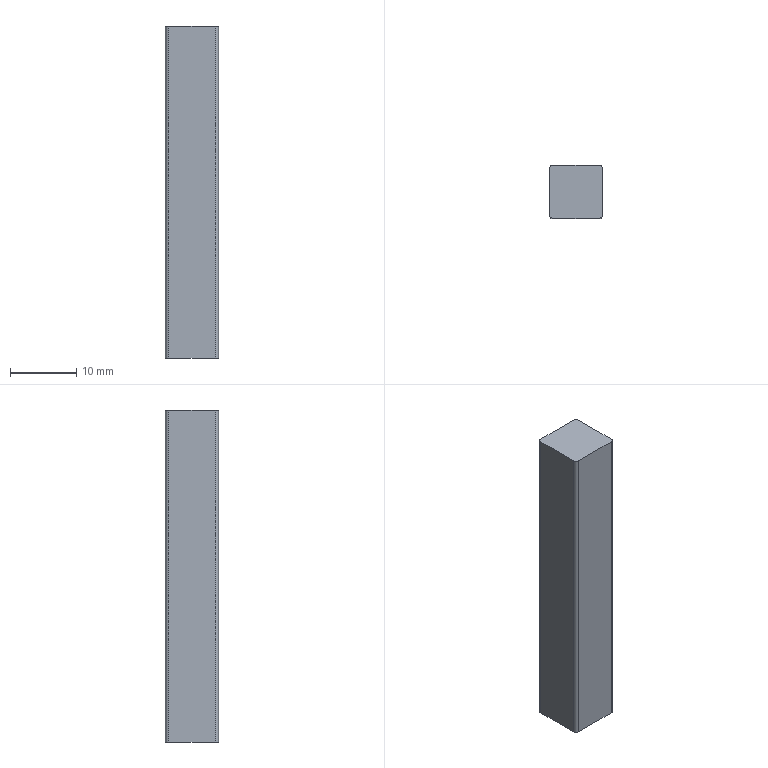Part | NX | features BREP 1 | 1 solid | 10 faces | box 8 x 8 x 50 mm | volume 3189 mm3 | plane 6 | cylinder 4 | commonest cylinder face diameters 1 x4
STEP:
#1=CARTESIAN_POINT('',(-3.5,4.,-40.6));
#2=VERTEX_POINT('',#1);
#3=CARTESIAN_POINT('',(-4.,3.5,-40.6));
#4=VERTEX_POINT('',#3);
#5=CARTESIAN_POINT('',(-3.5,3.5,-40.6));
#6=DIRECTION('',(0.,0.,1.));
#7=DIRECTION('',(1.,0.,0.));
#8=AXIS2_PLACEMENT_3D('',#5,#6,#7);
#9=CIRCLE('',#8,0.5);
#10=EDGE_CURVE('',#2,#4,#9,.T.);
#11=ORIENTED_EDGE('',*,*,#10,.F.);
#12=CARTESIAN_POINT('',(-3.5,4.,-90.6));
#13=VERTEX_POINT('',#12);
#14=CARTESIAN_POINT('',(-3.5,4.,-90.6));
#15=DIRECTION('',(0.,0.,1.));
#16=VECTOR('',#15,1000.);
#17=LINE('',#14,#16);
#18=EDGE_CURVE('',#13,#2,#17,.T.);
#19=ORIENTED_EDGE('',*,*,#18,.F.);
#20=CARTESIAN_POINT('',(-4.,3.5,-90.6));
#21=VERTEX_POINT('',#20);
#22=CARTESIAN_POINT('',(-3.5,3.5,-90.6));
#23=DIRECTION('',(0.,0.,1.));
#24=DIRECTION('',(1.,0.,0.));
#25=AXIS2_PLACEMENT_3D('',#22,#23,#24);
#26=CIRCLE('',#25,0.5);
#27=EDGE_CURVE('',#13,#21,#26,.T.);
#28=ORIENTED_EDGE('',*,*,#27,.T.);
#29=CARTESIAN_POINT('',(-4.,3.5,-90.6));
#30=DIRECTION('',(0.,0.,1.));
#31=VECTOR('',#30,1000.);
#32=LINE('',#29,#31);
#33=EDGE_CURVE('',#21,#4,#32,.T.);
#34=ORIENTED_EDGE('',*,*,#33,.T.);
#35=EDGE_LOOP('',(#11,#19,#28,#34));
#36=FACE_BOUND('',#35,.T.);
#37=CARTESIAN_POINT('',(-3.5,3.5,-90.6));
#38=DIRECTION('',(0.,0.,1.));
#39=DIRECTION('',(-1.,0.,0.));
#40=AXIS2_PLACEMENT_3D('',#37,#38,#39);
#41=CYLINDRICAL_SURFACE('',#40,0.5);
#42=ADVANCED_FACE('',(#36),#41,.T.);
#43=CARTESIAN_POINT('',(-4.,-3.5,-40.6));
#44=VERTEX_POINT('',#43);
#45=CARTESIAN_POINT('',(-4.,-3.5,-40.6));
#46=DIRECTION('',(0.,1.,0.));
#47=VECTOR('',#46,1000.);
#48=LINE('',#45,#47);
#49=EDGE_CURVE('',#44,#4,#48,.T.);
#50=ORIENTED_EDGE('',*,*,#49,.T.);
#51=ORIENTED_EDGE('',*,*,#33,.F.);
#52=CARTESIAN_POINT('',(-4.,-3.5,-90.6));
#53=VERTEX_POINT('',#52);
#54=CARTESIAN_POINT('',(-4.,-3.5,-90.6));
#55=DIRECTION('',(0.,1.,0.));
#56=VECTOR('',#55,1000.);
#57=LINE('',#54,#56);
#58=EDGE_CURVE('',#53,#21,#57,.T.);
#59=ORIENTED_EDGE('',*,*,#58,.F.);
#60=CARTESIAN_POINT('',(-4.,-3.5,-90.6));
#61=DIRECTION('',(0.,0.,1.));
#62=VECTOR('',#61,1000.);
#63=LINE('',#60,#62);
#64=EDGE_CURVE('',#53,#44,#63,.T.);
#65=ORIENTED_EDGE('',*,*,#64,.T.);
#66=EDGE_LOOP('',(#50,#51,#59,#65));
#67=FACE_BOUND('',#66,.T.);
#68=CARTESIAN_POINT('',(-4.,-3.5,-90.6));
#69=DIRECTION('',(1.,0.,0.));
#70=DIRECTION('',(0.,0.,1.));
#71=AXIS2_PLACEMENT_3D('',#68,#69,#70);
#72=PLANE('',#71);
#73=ADVANCED_FACE('',(#67),#72,.F.);
#74=CARTESIAN_POINT('',(-3.5,-4.,-40.6));
#75=VERTEX_POINT('',#74);
#76=CARTESIAN_POINT('',(-3.5,-3.5,-40.6));
#77=DIRECTION('',(0.,0.,1.));
#78=DIRECTION('',(1.,0.,0.));
#79=AXIS2_PLACEMENT_3D('',#76,#77,#78);
#80=CIRCLE('',#79,0.5);
#81=EDGE_CURVE('',#44,#75,#80,.T.);
#82=ORIENTED_EDGE('',*,*,#81,.F.);
#83=ORIENTED_EDGE('',*,*,#64,.F.);
#84=CARTESIAN_POINT('',(-3.5,-4.,-90.6));
#85=VERTEX_POINT('',#84);
#86=CARTESIAN_POINT('',(-3.5,-3.5,-90.6));
#87=DIRECTION('',(0.,0.,1.));
#88=DIRECTION('',(1.,0.,0.));
#89=AXIS2_PLACEMENT_3D('',#86,#87,#88);
#90=CIRCLE('',#89,0.5);
#91=EDGE_CURVE('',#53,#85,#90,.T.);
#92=ORIENTED_EDGE('',*,*,#91,.T.);
#93=CARTESIAN_POINT('',(-3.5,-4.,-90.6));
#94=DIRECTION('',(0.,0.,1.));
#95=VECTOR('',#94,1000.);
#96=LINE('',#93,#95);
#97=EDGE_CURVE('',#85,#75,#96,.T.);
#98=ORIENTED_EDGE('',*,*,#97,.T.);
#99=EDGE_LOOP('',(#82,#83,#92,#98));
#100=FACE_BOUND('',#99,.T.);
#101=CARTESIAN_POINT('',(-3.5,-3.5,-90.6));
#102=DIRECTION('',(0.,0.,1.));
#103=DIRECTION('',(-1.,0.,0.));
#104=AXIS2_PLACEMENT_3D('',#101,#102,#103);
#105=CYLINDRICAL_SURFACE('',#104,0.5);
#106=ADVANCED_FACE('',(#100),#105,.T.);
#107=CARTESIAN_POINT('',(3.5,-4.,-40.6));
#108=VERTEX_POINT('',#107);
#109=CARTESIAN_POINT('',(3.5,-4.,-40.6));
#110=DIRECTION('',(-1.,0.,0.));
#111=VECTOR('',#110,1000.);
#112=LINE('',#109,#111);
#113=EDGE_CURVE('',#108,#75,#112,.T.);
#114=ORIENTED_EDGE('',*,*,#113,.T.);
#115=ORIENTED_EDGE('',*,*,#97,.F.);
#116=CARTESIAN_POINT('',(3.5,-4.,-90.6));
#117=VERTEX_POINT('',#116);
#118=CARTESIAN_POINT('',(3.5,-4.,-90.6));
#119=DIRECTION('',(-1.,0.,0.));
#120=VECTOR('',#119,1000.);
#121=LINE('',#118,#120);
#122=EDGE_CURVE('',#117,#85,#121,.T.);
#123=ORIENTED_EDGE('',*,*,#122,.F.);
#124=CARTESIAN_POINT('',(3.5,-4.,-90.6));
#125=DIRECTION('',(0.,0.,1.));
#126=VECTOR('',#125,1000.);
#127=LINE('',#124,#126);
#128=EDGE_CURVE('',#117,#108,#127,.T.);
#129=ORIENTED_EDGE('',*,*,#128,.T.);
#130=EDGE_LOOP('',(#114,#115,#123,#129));
#131=FACE_BOUND('',#130,.T.);
#132=CARTESIAN_POINT('',(3.5,-4.,-90.6));
#133=DIRECTION('',(0.,1.,0.));
#134=DIRECTION('',(0.,0.,-1.));
#135=AXIS2_PLACEMENT_3D('',#132,#133,#134);
#136=PLANE('',#135);
#137=ADVANCED_FACE('',(#131),#136,.F.);
#138=CARTESIAN_POINT('',(4.,-3.5,-40.6));
#139=VERTEX_POINT('',#138);
#140=CARTESIAN_POINT('',(3.5,-3.5,-40.6));
#141=DIRECTION('',(0.,0.,1.));
#142=DIRECTION('',(1.,0.,0.));
#143=AXIS2_PLACEMENT_3D('',#140,#141,#142);
#144=CIRCLE('',#143,0.5);
#145=EDGE_CURVE('',#108,#139,#144,.T.);
#146=ORIENTED_EDGE('',*,*,#145,.F.);
#147=ORIENTED_EDGE('',*,*,#128,.F.);
#148=CARTESIAN_POINT('',(4.,-3.5,-90.6));
#149=VERTEX_POINT('',#148);
#150=CARTESIAN_POINT('',(3.5,-3.5,-90.6));
#151=DIRECTION('',(0.,0.,1.));
#152=DIRECTION('',(1.,0.,0.));
#153=AXIS2_PLACEMENT_3D('',#150,#151,#152);
#154=CIRCLE('',#153,0.5);
#155=EDGE_CURVE('',#117,#149,#154,.T.);
#156=ORIENTED_EDGE('',*,*,#155,.T.);
#157=CARTESIAN_POINT('',(4.,-3.5,-90.6));
#158=DIRECTION('',(0.,0.,1.));
#159=VECTOR('',#158,1000.);
#160=LINE('',#157,#159);
#161=EDGE_CURVE('',#149,#139,#160,.T.);
#162=ORIENTED_EDGE('',*,*,#161,.T.);
#163=EDGE_LOOP('',(#146,#147,#156,#162));
#164=FACE_BOUND('',#163,.T.);
#165=CARTESIAN_POINT('',(3.5,-3.5,-90.6));
#166=DIRECTION('',(0.,0.,1.));
#167=DIRECTION('',(-1.,0.,0.));
#168=AXIS2_PLACEMENT_3D('',#165,#166,#167);
#169=CYLINDRICAL_SURFACE('',#168,0.5);
#170=ADVANCED_FACE('',(#164),#169,.T.);
#171=CARTESIAN_POINT('',(4.,3.5,-40.6));
#172=VERTEX_POINT('',#171);
#173=CARTESIAN_POINT('',(4.,3.5,-40.6));
#174=DIRECTION('',(0.,-1.,0.));
#175=VECTOR('',#174,1000.);
#176=LINE('',#173,#175);
#177=EDGE_CURVE('',#172,#139,#176,.T.);
#178=ORIENTED_EDGE('',*,*,#177,.T.);
#179=ORIENTED_EDGE('',*,*,#161,.F.);
#180=CARTESIAN_POINT('',(4.,3.5,-90.6));
#181=VERTEX_POINT('',#180);
#182=CARTESIAN_POINT('',(4.,3.5,-90.6));
#183=DIRECTION('',(0.,-1.,0.));
#184=VECTOR('',#183,1000.);
#185=LINE('',#182,#184);
#186=EDGE_CURVE('',#181,#149,#185,.T.);
#187=ORIENTED_EDGE('',*,*,#186,.F.);
#188=CARTESIAN_POINT('',(4.,3.5,-90.6));
#189=DIRECTION('',(0.,0.,1.));
#190=VECTOR('',#189,1000.);
#191=LINE('',#188,#190);
#192=EDGE_CURVE('',#181,#172,#191,.T.);
#193=ORIENTED_EDGE('',*,*,#192,.T.);
#194=EDGE_LOOP('',(#178,#179,#187,#193));
#195=FACE_BOUND('',#194,.T.);
#196=CARTESIAN_POINT('',(4.,3.5,-90.6));
#197=DIRECTION('',(-1.,0.,0.));
#198=DIRECTION('',(0.,0.,-1.));
#199=AXIS2_PLACEMENT_3D('',#196,#197,#198);
#200=PLANE('',#199);
#201=ADVANCED_FACE('',(#195),#200,.F.);
#202=CARTESIAN_POINT('',(3.5,4.,-40.6));
#203=VERTEX_POINT('',#202);
#204=CARTESIAN_POINT('',(3.5,3.5,-40.6));
#205=DIRECTION('',(0.,0.,1.));
#206=DIRECTION('',(1.,0.,0.));
#207=AXIS2_PLACEMENT_3D('',#204,#205,#206);
#208=CIRCLE('',#207,0.5);
#209=EDGE_CURVE('',#172,#203,#208,.T.);
#210=ORIENTED_EDGE('',*,*,#209,.F.);
#211=ORIENTED_EDGE('',*,*,#192,.F.);
#212=CARTESIAN_POINT('',(3.5,4.,-90.6));
#213=VERTEX_POINT('',#212);
#214=CARTESIAN_POINT('',(3.5,3.5,-90.6));
#215=DIRECTION('',(0.,0.,1.));
#216=DIRECTION('',(1.,0.,0.));
#217=AXIS2_PLACEMENT_3D('',#214,#215,#216);
#218=CIRCLE('',#217,0.5);
#219=EDGE_CURVE('',#181,#213,#218,.T.);
#220=ORIENTED_EDGE('',*,*,#219,.T.);
#221=CARTESIAN_POINT('',(3.5,4.,-90.6));
#222=DIRECTION('',(0.,0.,1.));
#223=VECTOR('',#222,1000.);
#224=LINE('',#221,#223);
#225=EDGE_CURVE('',#213,#203,#224,.T.);
#226=ORIENTED_EDGE('',*,*,#225,.T.);
#227=EDGE_LOOP('',(#210,#211,#220,#226));
#228=FACE_BOUND('',#227,.T.);
#229=CARTESIAN_POINT('',(3.5,3.5,-90.6));
#230=DIRECTION('',(0.,0.,1.));
#231=DIRECTION('',(-1.,0.,0.));
#232=AXIS2_PLACEMENT_3D('',#229,#230,#231);
#233=CYLINDRICAL_SURFACE('',#232,0.5);
#234=ADVANCED_FACE('',(#228),#233,.T.);
#235=CARTESIAN_POINT('',(-3.5,4.,-40.6));
#236=DIRECTION('',(1.,0.,0.));
#237=VECTOR('',#236,1000.);
#238=LINE('',#235,#237);
#239=EDGE_CURVE('',#2,#203,#238,.T.);
#240=ORIENTED_EDGE('',*,*,#239,.T.);
#241=ORIENTED_EDGE('',*,*,#225,.F.);
#242=CARTESIAN_POINT('',(-3.5,4.,-90.6));
#243=DIRECTION('',(1.,0.,0.));
#244=VECTOR('',#243,1000.);
#245=LINE('',#242,#244);
#246=EDGE_CURVE('',#13,#213,#245,.T.);
#247=ORIENTED_EDGE('',*,*,#246,.F.);
#248=ORIENTED_EDGE('',*,*,#18,.T.);
#249=EDGE_LOOP('',(#240,#241,#247,#248));
#250=FACE_BOUND('',#249,.T.);
#251=CARTESIAN_POINT('',(-3.5,4.,-90.6));
#252=DIRECTION('',(0.,-1.,0.));
#253=DIRECTION('',(0.,0.,1.));
#254=AXIS2_PLACEMENT_3D('',#251,#252,#253);
#255=PLANE('',#254);
#256=ADVANCED_FACE('',(#250),#255,.F.);
#257=ORIENTED_EDGE('',*,*,#27,.F.);
#258=ORIENTED_EDGE('',*,*,#246,.T.);
#259=ORIENTED_EDGE('',*,*,#219,.F.);
#260=ORIENTED_EDGE('',*,*,#186,.T.);
#261=ORIENTED_EDGE('',*,*,#155,.F.);
#262=ORIENTED_EDGE('',*,*,#122,.T.);
#263=ORIENTED_EDGE('',*,*,#91,.F.);
#264=ORIENTED_EDGE('',*,*,#58,.T.);
#265=EDGE_LOOP('',(#257,#258,#259,#260,#261,#262,#263,#264));
#266=FACE_BOUND('',#265,.T.);
#267=CARTESIAN_POINT('',(-3.5,3.5,-90.6));
#268=DIRECTION('',(0.,0.,1.));
#269=DIRECTION('',(-1.,0.,0.));
#270=AXIS2_PLACEMENT_3D('',#267,#268,#269);
#271=PLANE('',#270);
#272=ADVANCED_FACE('',(#266),#271,.F.);
#273=ORIENTED_EDGE('',*,*,#10,.T.);
#274=ORIENTED_EDGE('',*,*,#49,.F.);
#275=ORIENTED_EDGE('',*,*,#81,.T.);
#276=ORIENTED_EDGE('',*,*,#113,.F.);
#277=ORIENTED_EDGE('',*,*,#145,.T.);
#278=ORIENTED_EDGE('',*,*,#177,.F.);
#279=ORIENTED_EDGE('',*,*,#209,.T.);
#280=ORIENTED_EDGE('',*,*,#239,.F.);
#281=EDGE_LOOP('',(#273,#274,#275,#276,#277,#278,#279,#280));
#282=FACE_BOUND('',#281,.T.);
#283=CARTESIAN_POINT('',(-3.5,3.5,-40.6));
#284=DIRECTION('',(0.,0.,1.));
#285=DIRECTION('',(-1.,0.,0.));
#286=AXIS2_PLACEMENT_3D('',#283,#284,#285);
#287=PLANE('',#286);
#288=ADVANCED_FACE('',(#282),#287,.T.);
#289=CLOSED_SHELL('',(#42,#73,#106,#137,#170,#201,#234,#256,#272,#288));
#290=MANIFOLD_SOLID_BREP('',#289);
#291=(LENGTH_UNIT()NAMED_UNIT(*)SI_UNIT(.MILLI.,.METRE.));
#292=UNCERTAINTY_MEASURE_WITH_UNIT(LENGTH_MEASURE(0.00001),#291,'','');
#293=(NAMED_UNIT(*)PLANE_ANGLE_UNIT()SI_UNIT($,.RADIAN.));
#294=(NAMED_UNIT(*)SI_UNIT($,.STERADIAN.)SOLID_ANGLE_UNIT());
#295=(GEOMETRIC_REPRESENTATION_CONTEXT(3)GLOBAL_UNCERTAINTY_ASSIGNED_CONTEXT((#292))GLOBAL_UNIT_ASSIGNED_CONTEXT((#291,#293,#294))REPRESENTATION_CONTEXT('',''));
#296=ADVANCED_BREP_SHAPE_REPRESENTATION('',(#290),#295);